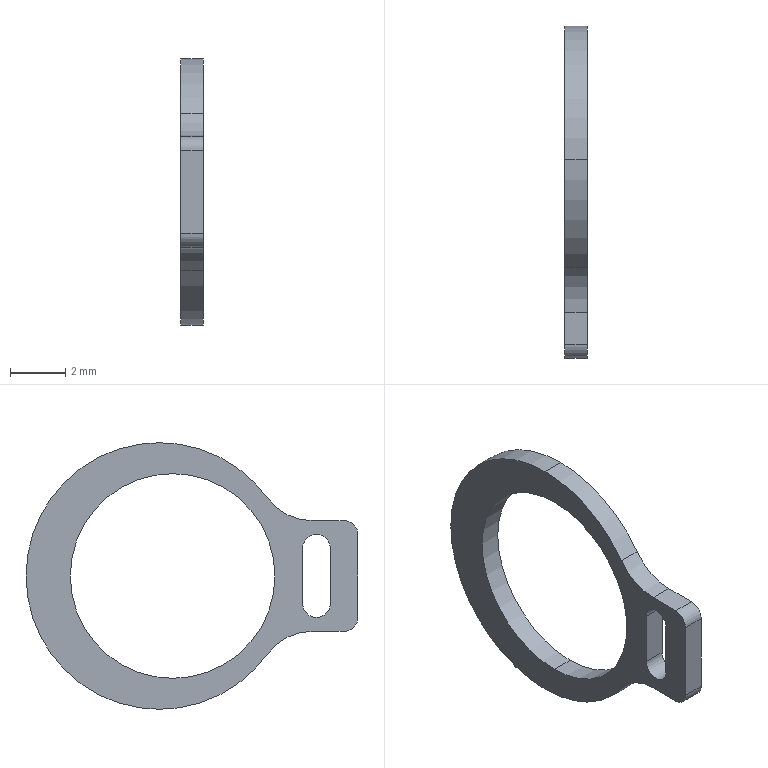Part | STEP file | 11-STWN811 | 1 solid | 19 faces | box 0.8 x 12 x 9.64 mm | volume 29.975 mm3 | cylinder 12 | plane 7 | commonest cylinder face diameters 1 x5 9.64 x3 4 x2 7.4 x2
STEP:
#1=CARTESIAN_POINT('',(0.4,0.,3.7));
#2=VERTEX_POINT('',#1);
#3=CARTESIAN_POINT('',(0.4,0.,-3.7));
#4=VERTEX_POINT('',#3);
#5=CARTESIAN_POINT('',(0.4,0.,0.));
#6=DIRECTION('',(1.,0.,0.));
#7=DIRECTION('',(0.,0.,-1.));
#8=AXIS2_PLACEMENT_3D('',#5,#6,#7);
#9=CIRCLE('',#8,3.7);
#10=EDGE_CURVE('',#2,#4,#9,.T.);
#11=ORIENTED_EDGE('',*,*,#10,.T.);
#12=CARTESIAN_POINT('',(-0.4,0.,-3.7));
#13=VERTEX_POINT('',#12);
#14=CARTESIAN_POINT('',(0.4,0.,-3.7));
#15=DIRECTION('',(-1.,0.,0.));
#16=VECTOR('',#15,1000.);
#17=LINE('',#14,#16);
#18=EDGE_CURVE('',#4,#13,#17,.T.);
#19=ORIENTED_EDGE('',*,*,#18,.T.);
#20=CARTESIAN_POINT('',(-0.4,0.,3.7));
#21=VERTEX_POINT('',#20);
#22=CARTESIAN_POINT('',(-0.4,0.,0.));
#23=DIRECTION('',(1.,0.,0.));
#24=DIRECTION('',(0.,0.,-1.));
#25=AXIS2_PLACEMENT_3D('',#22,#23,#24);
#26=CIRCLE('',#25,3.7);
#27=EDGE_CURVE('',#21,#13,#26,.T.);
#28=ORIENTED_EDGE('',*,*,#27,.F.);
#29=CARTESIAN_POINT('',(0.4,0.,3.7));
#30=DIRECTION('',(-1.,0.,0.));
#31=VECTOR('',#30,1000.);
#32=LINE('',#29,#31);
#33=EDGE_CURVE('',#2,#21,#32,.T.);
#34=ORIENTED_EDGE('',*,*,#33,.F.);
#35=EDGE_LOOP('',(#11,#19,#28,#34));
#36=FACE_OUTER_BOUND('',#35,.T.);
#37=CARTESIAN_POINT('',(0.4,0.,0.));
#38=DIRECTION('',(-1.,0.,0.));
#39=DIRECTION('',(0.,0.,1.));
#40=AXIS2_PLACEMENT_3D('',#37,#38,#39);
#41=CYLINDRICAL_SURFACE('',#40,3.7);
#42=ADVANCED_FACE('',(#36),#41,.F.);
#43=CARTESIAN_POINT('',(0.4,-4.7,1.));
#44=VERTEX_POINT('',#43);
#45=CARTESIAN_POINT('',(0.4,-5.2,1.5));
#46=VERTEX_POINT('',#45);
#47=CARTESIAN_POINT('',(0.4,-5.2,1.));
#48=DIRECTION('',(1.,0.,0.));
#49=DIRECTION('',(0.,0.,-1.));
#50=AXIS2_PLACEMENT_3D('',#47,#48,#49);
#51=CIRCLE('',#50,0.5);
#52=EDGE_CURVE('',#44,#46,#51,.T.);
#53=ORIENTED_EDGE('',*,*,#52,.T.);
#54=CARTESIAN_POINT('',(-0.4,-5.2,1.5));
#55=VERTEX_POINT('',#54);
#56=CARTESIAN_POINT('',(0.4,-5.2,1.5));
#57=DIRECTION('',(-1.,0.,0.));
#58=VECTOR('',#57,1000.);
#59=LINE('',#56,#58);
#60=EDGE_CURVE('',#46,#55,#59,.T.);
#61=ORIENTED_EDGE('',*,*,#60,.T.);
#62=CARTESIAN_POINT('',(-0.4,-4.7,1.));
#63=VERTEX_POINT('',#62);
#64=CARTESIAN_POINT('',(-0.4,-5.2,1.));
#65=DIRECTION('',(1.,0.,0.));
#66=DIRECTION('',(0.,0.,-1.));
#67=AXIS2_PLACEMENT_3D('',#64,#65,#66);
#68=CIRCLE('',#67,0.5);
#69=EDGE_CURVE('',#63,#55,#68,.T.);
#70=ORIENTED_EDGE('',*,*,#69,.F.);
#71=CARTESIAN_POINT('',(0.4,-4.7,1.));
#72=DIRECTION('',(-1.,0.,0.));
#73=VECTOR('',#72,1000.);
#74=LINE('',#71,#73);
#75=EDGE_CURVE('',#44,#63,#74,.T.);
#76=ORIENTED_EDGE('',*,*,#75,.F.);
#77=EDGE_LOOP('',(#53,#61,#70,#76));
#78=FACE_OUTER_BOUND('',#77,.T.);
#79=CARTESIAN_POINT('',(0.4,-5.2,1.));
#80=DIRECTION('',(-1.,0.,0.));
#81=DIRECTION('',(0.,0.,1.));
#82=AXIS2_PLACEMENT_3D('',#79,#80,#81);
#83=CYLINDRICAL_SURFACE('',#82,0.5);
#84=ADVANCED_FACE('',(#78),#83,.F.);
#85=CARTESIAN_POINT('',(0.4,0.48,-4.82));
#86=VERTEX_POINT('',#85);
#87=CARTESIAN_POINT('',(0.4,0.48,4.82));
#88=VERTEX_POINT('',#87);
#89=CARTESIAN_POINT('',(0.4,0.48,0.));
#90=DIRECTION('',(1.,0.,0.));
#91=DIRECTION('',(0.,0.,-1.));
#92=AXIS2_PLACEMENT_3D('',#89,#90,#91);
#93=CIRCLE('',#92,4.82);
#94=EDGE_CURVE('',#86,#88,#93,.T.);
#95=ORIENTED_EDGE('',*,*,#94,.F.);
#96=CARTESIAN_POINT('',(-0.4,0.48,-4.82));
#97=VERTEX_POINT('',#96);
#98=CARTESIAN_POINT('',(0.4,0.48,-4.82));
#99=DIRECTION('',(-1.,0.,0.));
#100=VECTOR('',#99,1000.);
#101=LINE('',#98,#100);
#102=EDGE_CURVE('',#86,#97,#101,.T.);
#103=ORIENTED_EDGE('',*,*,#102,.T.);
#104=CARTESIAN_POINT('',(-0.4,0.48,4.82));
#105=VERTEX_POINT('',#104);
#106=CARTESIAN_POINT('',(-0.4,0.48,0.));
#107=DIRECTION('',(1.,0.,0.));
#108=DIRECTION('',(0.,0.,-1.));
#109=AXIS2_PLACEMENT_3D('',#106,#107,#108);
#110=CIRCLE('',#109,4.82);
#111=EDGE_CURVE('',#97,#105,#110,.T.);
#112=ORIENTED_EDGE('',*,*,#111,.T.);
#113=CARTESIAN_POINT('',(0.4,0.48,4.82));
#114=DIRECTION('',(-1.,0.,0.));
#115=VECTOR('',#114,1000.);
#116=LINE('',#113,#115);
#117=EDGE_CURVE('',#88,#105,#116,.T.);
#118=ORIENTED_EDGE('',*,*,#117,.F.);
#119=EDGE_LOOP('',(#95,#103,#112,#118));
#120=FACE_OUTER_BOUND('',#119,.T.);
#121=CARTESIAN_POINT('',(0.4,0.48,0.));
#122=DIRECTION('',(-1.,0.,0.));
#123=DIRECTION('',(0.,0.,1.));
#124=AXIS2_PLACEMENT_3D('',#121,#122,#123);
#125=CYLINDRICAL_SURFACE('',#124,4.82);
#126=ADVANCED_FACE('',(#120),#125,.T.);
#127=CARTESIAN_POINT('',(0.4,-3.424,2.827));
#128=VERTEX_POINT('',#127);
#129=CARTESIAN_POINT('',(0.4,0.48,0.));
#130=DIRECTION('',(1.,0.,0.));
#131=DIRECTION('',(0.,0.,-1.));
#132=AXIS2_PLACEMENT_3D('',#129,#130,#131);
#133=CIRCLE('',#132,4.82);
#134=EDGE_CURVE('',#88,#128,#133,.T.);
#135=ORIENTED_EDGE('',*,*,#134,.F.);
#136=ORIENTED_EDGE('',*,*,#117,.T.);
#137=CARTESIAN_POINT('',(-0.4,-3.424,2.827));
#138=VERTEX_POINT('',#137);
#139=CARTESIAN_POINT('',(-0.4,0.48,0.));
#140=DIRECTION('',(1.,0.,0.));
#141=DIRECTION('',(0.,0.,-1.));
#142=AXIS2_PLACEMENT_3D('',#139,#140,#141);
#143=CIRCLE('',#142,4.82);
#144=EDGE_CURVE('',#105,#138,#143,.T.);
#145=ORIENTED_EDGE('',*,*,#144,.T.);
#146=CARTESIAN_POINT('',(0.4,-3.424,2.827));
#147=DIRECTION('',(-1.,0.,0.));
#148=VECTOR('',#147,1000.);
#149=LINE('',#146,#148);
#150=EDGE_CURVE('',#128,#138,#149,.T.);
#151=ORIENTED_EDGE('',*,*,#150,.F.);
#152=EDGE_LOOP('',(#135,#136,#145,#151));
#153=FACE_OUTER_BOUND('',#152,.T.);
#154=CARTESIAN_POINT('',(0.4,0.48,0.));
#155=DIRECTION('',(-1.,0.,0.));
#156=DIRECTION('',(0.,0.,1.));
#157=AXIS2_PLACEMENT_3D('',#154,#155,#156);
#158=CYLINDRICAL_SURFACE('',#157,4.82);
#159=ADVANCED_FACE('',(#153),#158,.T.);
#160=ORIENTED_EDGE('',*,*,#52,.F.);
#161=CARTESIAN_POINT('',(0.4,-4.7,-1.));
#162=VERTEX_POINT('',#161);
#163=CARTESIAN_POINT('',(0.4,-4.7,-1.));
#164=DIRECTION('',(0.,0.,1.));
#165=VECTOR('',#164,1000.);
#166=LINE('',#163,#165);
#167=EDGE_CURVE('',#162,#44,#166,.T.);
#168=ORIENTED_EDGE('',*,*,#167,.F.);
#169=CARTESIAN_POINT('',(0.4,-5.7,-1.));
#170=VERTEX_POINT('',#169);
#171=CARTESIAN_POINT('',(0.4,-5.2,-1.));
#172=DIRECTION('',(1.,0.,0.));
#173=DIRECTION('',(0.,0.,-1.));
#174=AXIS2_PLACEMENT_3D('',#171,#172,#173);
#175=CIRCLE('',#174,0.5);
#176=EDGE_CURVE('',#170,#162,#175,.T.);
#177=ORIENTED_EDGE('',*,*,#176,.F.);
#178=CARTESIAN_POINT('',(0.4,-5.7,1.));
#179=VERTEX_POINT('',#178);
#180=CARTESIAN_POINT('',(0.4,-5.7,1.));
#181=DIRECTION('',(0.,0.,-1.));
#182=VECTOR('',#181,1000.);
#183=LINE('',#180,#182);
#184=EDGE_CURVE('',#179,#170,#183,.T.);
#185=ORIENTED_EDGE('',*,*,#184,.F.);
#186=CARTESIAN_POINT('',(0.4,-5.2,1.));
#187=DIRECTION('',(1.,0.,0.));
#188=DIRECTION('',(0.,0.,-1.));
#189=AXIS2_PLACEMENT_3D('',#186,#187,#188);
#190=CIRCLE('',#189,0.5);
#191=EDGE_CURVE('',#46,#179,#190,.T.);
#192=ORIENTED_EDGE('',*,*,#191,.F.);
#193=EDGE_LOOP('',(#160,#168,#177,#185,#192));
#194=FACE_BOUND('',#193,.T.);
#195=CARTESIAN_POINT('',(0.4,-5.044,-2.));
#196=VERTEX_POINT('',#195);
#197=CARTESIAN_POINT('',(0.4,-3.424,-2.827));
#198=VERTEX_POINT('',#197);
#199=CARTESIAN_POINT('',(0.4,-5.044,-4.));
#200=DIRECTION('',(-1.,0.,0.));
#201=DIRECTION('',(0.,0.,1.));
#202=AXIS2_PLACEMENT_3D('',#199,#200,#201);
#203=CIRCLE('',#202,2.);
#204=EDGE_CURVE('',#196,#198,#203,.T.);
#205=ORIENTED_EDGE('',*,*,#204,.T.);
#206=CARTESIAN_POINT('',(0.4,0.48,0.));
#207=DIRECTION('',(1.,0.,0.));
#208=DIRECTION('',(0.,0.,-1.));
#209=AXIS2_PLACEMENT_3D('',#206,#207,#208);
#210=CIRCLE('',#209,4.82);
#211=EDGE_CURVE('',#198,#86,#210,.T.);
#212=ORIENTED_EDGE('',*,*,#211,.T.);
#213=ORIENTED_EDGE('',*,*,#94,.T.);
#214=ORIENTED_EDGE('',*,*,#134,.T.);
#215=CARTESIAN_POINT('',(0.4,-5.044,2.));
#216=VERTEX_POINT('',#215);
#217=CARTESIAN_POINT('',(0.4,-5.044,4.));
#218=DIRECTION('',(-1.,0.,0.));
#219=DIRECTION('',(0.,0.,1.));
#220=AXIS2_PLACEMENT_3D('',#217,#218,#219);
#221=CIRCLE('',#220,2.);
#222=EDGE_CURVE('',#128,#216,#221,.T.);
#223=ORIENTED_EDGE('',*,*,#222,.T.);
#224=CARTESIAN_POINT('',(0.4,-6.2,2.));
#225=VERTEX_POINT('',#224);
#226=CARTESIAN_POINT('',(0.4,-5.044,2.));
#227=DIRECTION('',(0.,-1.,0.));
#228=VECTOR('',#227,1000.);
#229=LINE('',#226,#228);
#230=EDGE_CURVE('',#216,#225,#229,.T.);
#231=ORIENTED_EDGE('',*,*,#230,.T.);
#232=CARTESIAN_POINT('',(0.4,-6.7,1.5));
#233=VERTEX_POINT('',#232);
#234=CARTESIAN_POINT('',(0.4,-6.2,1.5));
#235=DIRECTION('',(1.,0.,0.));
#236=DIRECTION('',(0.,0.,-1.));
#237=AXIS2_PLACEMENT_3D('',#234,#235,#236);
#238=CIRCLE('',#237,0.5);
#239=EDGE_CURVE('',#225,#233,#238,.T.);
#240=ORIENTED_EDGE('',*,*,#239,.T.);
#241=CARTESIAN_POINT('',(0.4,-6.7,-1.5));
#242=VERTEX_POINT('',#241);
#243=CARTESIAN_POINT('',(0.4,-6.7,1.5));
#244=DIRECTION('',(0.,0.,-1.));
#245=VECTOR('',#244,1000.);
#246=LINE('',#243,#245);
#247=EDGE_CURVE('',#233,#242,#246,.T.);
#248=ORIENTED_EDGE('',*,*,#247,.T.);
#249=CARTESIAN_POINT('',(0.4,-6.2,-2.));
#250=VERTEX_POINT('',#249);
#251=CARTESIAN_POINT('',(0.4,-6.2,-1.5));
#252=DIRECTION('',(1.,0.,0.));
#253=DIRECTION('',(0.,0.,-1.));
#254=AXIS2_PLACEMENT_3D('',#251,#252,#253);
#255=CIRCLE('',#254,0.5);
#256=EDGE_CURVE('',#242,#250,#255,.T.);
#257=ORIENTED_EDGE('',*,*,#256,.T.);
#258=CARTESIAN_POINT('',(0.4,-6.2,-2.));
#259=DIRECTION('',(0.,1.,0.));
#260=VECTOR('',#259,1000.);
#261=LINE('',#258,#260);
#262=EDGE_CURVE('',#250,#196,#261,.T.);
#263=ORIENTED_EDGE('',*,*,#262,.T.);
#264=EDGE_LOOP('',(#205,#212,#213,#214,#223,#231,#240,#248,#257,#263));
#265=FACE_OUTER_BOUND('',#264,.T.);
#266=ORIENTED_EDGE('',*,*,#10,.F.);
#267=CARTESIAN_POINT('',(0.4,0.,0.));
#268=DIRECTION('',(1.,0.,0.));
#269=DIRECTION('',(0.,0.,-1.));
#270=AXIS2_PLACEMENT_3D('',#267,#268,#269);
#271=CIRCLE('',#270,3.7);
#272=EDGE_CURVE('',#4,#2,#271,.T.);
#273=ORIENTED_EDGE('',*,*,#272,.F.);
#274=EDGE_LOOP('',(#266,#273));
#275=FACE_BOUND('',#274,.T.);
#276=CARTESIAN_POINT('',(0.4,-5.044,-4.));
#277=DIRECTION('',(-1.,0.,0.));
#278=DIRECTION('',(0.,0.,1.));
#279=AXIS2_PLACEMENT_3D('',#276,#277,#278);
#280=PLANE('',#279);
#281=ADVANCED_FACE('',(#194,#265,#275),#280,.F.);
#282=CARTESIAN_POINT('',(-0.4,-5.044,-2.));
#283=VERTEX_POINT('',#282);
#284=CARTESIAN_POINT('',(0.4,-5.044,-2.));
#285=DIRECTION('',(-1.,0.,0.));
#286=VECTOR('',#285,1000.);
#287=LINE('',#284,#286);
#288=EDGE_CURVE('',#196,#283,#287,.T.);
#289=ORIENTED_EDGE('',*,*,#288,.T.);
#290=CARTESIAN_POINT('',(-0.4,-3.424,-2.827));
#291=VERTEX_POINT('',#290);
#292=CARTESIAN_POINT('',(-0.4,-5.044,-4.));
#293=DIRECTION('',(-1.,0.,0.));
#294=DIRECTION('',(0.,0.,1.));
#295=AXIS2_PLACEMENT_3D('',#292,#293,#294);
#296=CIRCLE('',#295,2.);
#297=EDGE_CURVE('',#283,#291,#296,.T.);
#298=ORIENTED_EDGE('',*,*,#297,.T.);
#299=CARTESIAN_POINT('',(0.4,-3.424,-2.827));
#300=DIRECTION('',(-1.,0.,0.));
#301=VECTOR('',#300,1000.);
#302=LINE('',#299,#301);
#303=EDGE_CURVE('',#198,#291,#302,.T.);
#304=ORIENTED_EDGE('',*,*,#303,.F.);
#305=ORIENTED_EDGE('',*,*,#204,.F.);
#306=EDGE_LOOP('',(#289,#298,#304,#305));
#307=FACE_OUTER_BOUND('',#306,.T.);
#308=CARTESIAN_POINT('',(0.4,-5.044,-4.));
#309=DIRECTION('',(-1.,0.,0.));
#310=DIRECTION('',(0.,0.,1.));
#311=AXIS2_PLACEMENT_3D('',#308,#309,#310);
#312=CYLINDRICAL_SURFACE('',#311,2.);
#313=ADVANCED_FACE('',(#307),#312,.F.);
#314=ORIENTED_EDGE('',*,*,#102,.F.);
#315=ORIENTED_EDGE('',*,*,#211,.F.);
#316=ORIENTED_EDGE('',*,*,#303,.T.);
#317=CARTESIAN_POINT('',(-0.4,0.48,0.));
#318=DIRECTION('',(1.,0.,0.));
#319=DIRECTION('',(0.,0.,-1.));
#320=AXIS2_PLACEMENT_3D('',#317,#318,#319);
#321=CIRCLE('',#320,4.82);
#322=EDGE_CURVE('',#291,#97,#321,.T.);
#323=ORIENTED_EDGE('',*,*,#322,.T.);
#324=EDGE_LOOP('',(#314,#315,#316,#323));
#325=FACE_OUTER_BOUND('',#324,.T.);
#326=CARTESIAN_POINT('',(0.4,0.48,0.));
#327=DIRECTION('',(-1.,0.,0.));
#328=DIRECTION('',(0.,0.,1.));
#329=AXIS2_PLACEMENT_3D('',#326,#327,#328);
#330=CYLINDRICAL_SURFACE('',#329,4.82);
#331=ADVANCED_FACE('',(#325),#330,.T.);
#332=ORIENTED_EDGE('',*,*,#150,.T.);
#333=CARTESIAN_POINT('',(-0.4,-5.044,2.));
#334=VERTEX_POINT('',#333);
#335=CARTESIAN_POINT('',(-0.4,-5.044,4.));
#336=DIRECTION('',(-1.,0.,0.));
#337=DIRECTION('',(0.,0.,1.));
#338=AXIS2_PLACEMENT_3D('',#335,#336,#337);
#339=CIRCLE('',#338,2.);
#340=EDGE_CURVE('',#138,#334,#339,.T.);
#341=ORIENTED_EDGE('',*,*,#340,.T.);
#342=CARTESIAN_POINT('',(0.4,-5.044,2.));
#343=DIRECTION('',(-1.,0.,0.));
#344=VECTOR('',#343,1000.);
#345=LINE('',#342,#344);
#346=EDGE_CURVE('',#216,#334,#345,.T.);
#347=ORIENTED_EDGE('',*,*,#346,.F.);
#348=ORIENTED_EDGE('',*,*,#222,.F.);
#349=EDGE_LOOP('',(#332,#341,#347,#348));
#350=FACE_OUTER_BOUND('',#349,.T.);
#351=CARTESIAN_POINT('',(0.4,-5.044,4.));
#352=DIRECTION('',(-1.,0.,0.));
#353=DIRECTION('',(0.,0.,1.));
#354=AXIS2_PLACEMENT_3D('',#351,#352,#353);
#355=CYLINDRICAL_SURFACE('',#354,2.);
#356=ADVANCED_FACE('',(#350),#355,.F.);
#357=ORIENTED_EDGE('',*,*,#346,.T.);
#358=CARTESIAN_POINT('',(-0.4,-6.2,2.));
#359=VERTEX_POINT('',#358);
#360=CARTESIAN_POINT('',(-0.4,-5.044,2.));
#361=DIRECTION('',(0.,-1.,0.));
#362=VECTOR('',#361,1000.);
#363=LINE('',#360,#362);
#364=EDGE_CURVE('',#334,#359,#363,.T.);
#365=ORIENTED_EDGE('',*,*,#364,.T.);
#366=CARTESIAN_POINT('',(0.4,-6.2,2.));
#367=DIRECTION('',(-1.,0.,0.));
#368=VECTOR('',#367,1000.);
#369=LINE('',#366,#368);
#370=EDGE_CURVE('',#225,#359,#369,.T.);
#371=ORIENTED_EDGE('',*,*,#370,.F.);
#372=ORIENTED_EDGE('',*,*,#230,.F.);
#373=EDGE_LOOP('',(#357,#365,#371,#372));
#374=FACE_OUTER_BOUND('',#373,.T.);
#375=CARTESIAN_POINT('',(0.4,-5.044,2.));
#376=DIRECTION('',(0.,0.,-1.));
#377=DIRECTION('',(-1.,0.,0.));
#378=AXIS2_PLACEMENT_3D('',#375,#376,#377);
#379=PLANE('',#378);
#380=ADVANCED_FACE('',(#374),#379,.F.);
#381=ORIENTED_EDGE('',*,*,#370,.T.);
#382=CARTESIAN_POINT('',(-0.4,-6.7,1.5));
#383=VERTEX_POINT('',#382);
#384=CARTESIAN_POINT('',(-0.4,-6.2,1.5));
#385=DIRECTION('',(1.,0.,0.));
#386=DIRECTION('',(0.,0.,-1.));
#387=AXIS2_PLACEMENT_3D('',#384,#385,#386);
#388=CIRCLE('',#387,0.5);
#389=EDGE_CURVE('',#359,#383,#388,.T.);
#390=ORIENTED_EDGE('',*,*,#389,.T.);
#391=CARTESIAN_POINT('',(0.4,-6.7,1.5));
#392=DIRECTION('',(-1.,0.,0.));
#393=VECTOR('',#392,1000.);
#394=LINE('',#391,#393);
#395=EDGE_CURVE('',#233,#383,#394,.T.);
#396=ORIENTED_EDGE('',*,*,#395,.F.);
#397=ORIENTED_EDGE('',*,*,#239,.F.);
#398=EDGE_LOOP('',(#381,#390,#396,#397));
#399=FACE_OUTER_BOUND('',#398,.T.);
#400=CARTESIAN_POINT('',(0.4,-6.2,1.5));
#401=DIRECTION('',(-1.,0.,0.));
#402=DIRECTION('',(0.,0.,1.));
#403=AXIS2_PLACEMENT_3D('',#400,#401,#402);
#404=CYLINDRICAL_SURFACE('',#403,0.5);
#405=ADVANCED_FACE('',(#399),#404,.T.);
#406=ORIENTED_EDGE('',*,*,#395,.T.);
#407=CARTESIAN_POINT('',(-0.4,-6.7,-1.5));
#408=VERTEX_POINT('',#407);
#409=CARTESIAN_POINT('',(-0.4,-6.7,1.5));
#410=DIRECTION('',(0.,0.,-1.));
#411=VECTOR('',#410,1000.);
#412=LINE('',#409,#411);
#413=EDGE_CURVE('',#383,#408,#412,.T.);
#414=ORIENTED_EDGE('',*,*,#413,.T.);
#415=CARTESIAN_POINT('',(0.4,-6.7,-1.5));
#416=DIRECTION('',(-1.,0.,0.));
#417=VECTOR('',#416,1000.);
#418=LINE('',#415,#417);
#419=EDGE_CURVE('',#242,#408,#418,.T.);
#420=ORIENTED_EDGE('',*,*,#419,.F.);
#421=ORIENTED_EDGE('',*,*,#247,.F.);
#422=EDGE_LOOP('',(#406,#414,#420,#421));
#423=FACE_OUTER_BOUND('',#422,.T.);
#424=CARTESIAN_POINT('',(0.4,-6.7,1.5));
#425=DIRECTION('',(0.,1.,0.));
#426=DIRECTION('',(0.,0.,1.));
#427=AXIS2_PLACEMENT_3D('',#424,#425,#426);
#428=PLANE('',#427);
#429=ADVANCED_FACE('',(#423),#428,.F.);
#430=ORIENTED_EDGE('',*,*,#419,.T.);
#431=CARTESIAN_POINT('',(-0.4,-6.2,-2.));
#432=VERTEX_POINT('',#431);
#433=CARTESIAN_POINT('',(-0.4,-6.2,-1.5));
#434=DIRECTION('',(1.,0.,0.));
#435=DIRECTION('',(0.,0.,-1.));
#436=AXIS2_PLACEMENT_3D('',#433,#434,#435);
#437=CIRCLE('',#436,0.5);
#438=EDGE_CURVE('',#408,#432,#437,.T.);
#439=ORIENTED_EDGE('',*,*,#438,.T.);
#440=CARTESIAN_POINT('',(0.4,-6.2,-2.));
#441=DIRECTION('',(-1.,0.,0.));
#442=VECTOR('',#441,1000.);
#443=LINE('',#440,#442);
#444=EDGE_CURVE('',#250,#432,#443,.T.);
#445=ORIENTED_EDGE('',*,*,#444,.F.);
#446=ORIENTED_EDGE('',*,*,#256,.F.);
#447=EDGE_LOOP('',(#430,#439,#445,#446));
#448=FACE_OUTER_BOUND('',#447,.T.);
#449=CARTESIAN_POINT('',(0.4,-6.2,-1.5));
#450=DIRECTION('',(-1.,0.,0.));
#451=DIRECTION('',(0.,0.,1.));
#452=AXIS2_PLACEMENT_3D('',#449,#450,#451);
#453=CYLINDRICAL_SURFACE('',#452,0.5);
#454=ADVANCED_FACE('',(#448),#453,.T.);
#455=ORIENTED_EDGE('',*,*,#444,.T.);
#456=CARTESIAN_POINT('',(-0.4,-6.2,-2.));
#457=DIRECTION('',(0.,1.,0.));
#458=VECTOR('',#457,1000.);
#459=LINE('',#456,#458);
#460=EDGE_CURVE('',#432,#283,#459,.T.);
#461=ORIENTED_EDGE('',*,*,#460,.T.);
#462=ORIENTED_EDGE('',*,*,#288,.F.);
#463=ORIENTED_EDGE('',*,*,#262,.F.);
#464=EDGE_LOOP('',(#455,#461,#462,#463));
#465=FACE_OUTER_BOUND('',#464,.T.);
#466=CARTESIAN_POINT('',(0.4,-6.2,-2.));
#467=DIRECTION('',(0.,0.,1.));
#468=DIRECTION('',(1.,0.,0.));
#469=AXIS2_PLACEMENT_3D('',#466,#467,#468);
#470=PLANE('',#469);
#471=ADVANCED_FACE('',(#465),#470,.F.);
#472=ORIENTED_EDGE('',*,*,#60,.F.);
#473=ORIENTED_EDGE('',*,*,#191,.T.);
#474=CARTESIAN_POINT('',(-0.4,-5.7,1.));
#475=VERTEX_POINT('',#474);
#476=CARTESIAN_POINT('',(0.4,-5.7,1.));
#477=DIRECTION('',(-1.,0.,0.));
#478=VECTOR('',#477,1000.);
#479=LINE('',#476,#478);
#480=EDGE_CURVE('',#179,#475,#479,.T.);
#481=ORIENTED_EDGE('',*,*,#480,.T.);
#482=CARTESIAN_POINT('',(-0.4,-5.2,1.));
#483=DIRECTION('',(1.,0.,0.));
#484=DIRECTION('',(0.,0.,-1.));
#485=AXIS2_PLACEMENT_3D('',#482,#483,#484);
#486=CIRCLE('',#485,0.5);
#487=EDGE_CURVE('',#55,#475,#486,.T.);
#488=ORIENTED_EDGE('',*,*,#487,.F.);
#489=EDGE_LOOP('',(#472,#473,#481,#488));
#490=FACE_OUTER_BOUND('',#489,.T.);
#491=CARTESIAN_POINT('',(0.4,-5.2,1.));
#492=DIRECTION('',(-1.,0.,0.));
#493=DIRECTION('',(0.,0.,1.));
#494=AXIS2_PLACEMENT_3D('',#491,#492,#493);
#495=CYLINDRICAL_SURFACE('',#494,0.5);
#496=ADVANCED_FACE('',(#490),#495,.F.);
#497=CARTESIAN_POINT('',(-0.4,-5.7,-1.));
#498=VERTEX_POINT('',#497);
#499=CARTESIAN_POINT('',(0.4,-5.7,-1.));
#500=DIRECTION('',(-1.,0.,0.));
#501=VECTOR('',#500,1000.);
#502=LINE('',#499,#501);
#503=EDGE_CURVE('',#170,#498,#502,.T.);
#504=ORIENTED_EDGE('',*,*,#503,.T.);
#505=CARTESIAN_POINT('',(-0.4,-5.7,1.));
#506=DIRECTION('',(0.,0.,-1.));
#507=VECTOR('',#506,1000.);
#508=LINE('',#505,#507);
#509=EDGE_CURVE('',#475,#498,#508,.T.);
#510=ORIENTED_EDGE('',*,*,#509,.F.);
#511=ORIENTED_EDGE('',*,*,#480,.F.);
#512=ORIENTED_EDGE('',*,*,#184,.T.);
#513=EDGE_LOOP('',(#504,#510,#511,#512));
#514=FACE_OUTER_BOUND('',#513,.T.);
#515=CARTESIAN_POINT('',(0.4,-5.7,1.));
#516=DIRECTION('',(0.,1.,0.));
#517=DIRECTION('',(0.,0.,1.));
#518=AXIS2_PLACEMENT_3D('',#515,#516,#517);
#519=PLANE('',#518);
#520=ADVANCED_FACE('',(#514),#519,.T.);
#521=CARTESIAN_POINT('',(-0.4,-4.7,-1.));
#522=VERTEX_POINT('',#521);
#523=CARTESIAN_POINT('',(0.4,-4.7,-1.));
#524=DIRECTION('',(-1.,0.,0.));
#525=VECTOR('',#524,1000.);
#526=LINE('',#523,#525);
#527=EDGE_CURVE('',#162,#522,#526,.T.);
#528=ORIENTED_EDGE('',*,*,#527,.T.);
#529=CARTESIAN_POINT('',(-0.4,-5.2,-1.));
#530=DIRECTION('',(1.,0.,0.));
#531=DIRECTION('',(0.,0.,-1.));
#532=AXIS2_PLACEMENT_3D('',#529,#530,#531);
#533=CIRCLE('',#532,0.5);
#534=EDGE_CURVE('',#498,#522,#533,.T.);
#535=ORIENTED_EDGE('',*,*,#534,.F.);
#536=ORIENTED_EDGE('',*,*,#503,.F.);
#537=ORIENTED_EDGE('',*,*,#176,.T.);
#538=EDGE_LOOP('',(#528,#535,#536,#537));
#539=FACE_OUTER_BOUND('',#538,.T.);
#540=CARTESIAN_POINT('',(0.4,-5.2,-1.));
#541=DIRECTION('',(-1.,0.,0.));
#542=DIRECTION('',(0.,0.,1.));
#543=AXIS2_PLACEMENT_3D('',#540,#541,#542);
#544=CYLINDRICAL_SURFACE('',#543,0.5);
#545=ADVANCED_FACE('',(#539),#544,.F.);
#546=ORIENTED_EDGE('',*,*,#75,.T.);
#547=CARTESIAN_POINT('',(-0.4,-4.7,-1.));
#548=DIRECTION('',(0.,0.,1.));
#549=VECTOR('',#548,1000.);
#550=LINE('',#547,#549);
#551=EDGE_CURVE('',#522,#63,#550,.T.);
#552=ORIENTED_EDGE('',*,*,#551,.F.);
#553=ORIENTED_EDGE('',*,*,#527,.F.);
#554=ORIENTED_EDGE('',*,*,#167,.T.);
#555=EDGE_LOOP('',(#546,#552,#553,#554));
#556=FACE_OUTER_BOUND('',#555,.T.);
#557=CARTESIAN_POINT('',(0.4,-4.7,-1.));
#558=DIRECTION('',(0.,-1.,0.));
#559=DIRECTION('',(0.,0.,-1.));
#560=AXIS2_PLACEMENT_3D('',#557,#558,#559);
#561=PLANE('',#560);
#562=ADVANCED_FACE('',(#556),#561,.T.);
#563=ORIENTED_EDGE('',*,*,#18,.F.);
#564=ORIENTED_EDGE('',*,*,#272,.T.);
#565=ORIENTED_EDGE('',*,*,#33,.T.);
#566=CARTESIAN_POINT('',(-0.4,0.,0.));
#567=DIRECTION('',(1.,0.,0.));
#568=DIRECTION('',(0.,0.,-1.));
#569=AXIS2_PLACEMENT_3D('',#566,#567,#568);
#570=CIRCLE('',#569,3.7);
#571=EDGE_CURVE('',#13,#21,#570,.T.);
#572=ORIENTED_EDGE('',*,*,#571,.F.);
#573=EDGE_LOOP('',(#563,#564,#565,#572));
#574=FACE_OUTER_BOUND('',#573,.T.);
#575=CARTESIAN_POINT('',(0.4,0.,0.));
#576=DIRECTION('',(-1.,0.,0.));
#577=DIRECTION('',(0.,0.,1.));
#578=AXIS2_PLACEMENT_3D('',#575,#576,#577);
#579=CYLINDRICAL_SURFACE('',#578,3.7);
#580=ADVANCED_FACE('',(#574),#579,.F.);
#581=ORIENTED_EDGE('',*,*,#27,.T.);
#582=ORIENTED_EDGE('',*,*,#571,.T.);
#583=EDGE_LOOP('',(#581,#582));
#584=FACE_BOUND('',#583,.T.);
#585=ORIENTED_EDGE('',*,*,#69,.T.);
#586=ORIENTED_EDGE('',*,*,#487,.T.);
#587=ORIENTED_EDGE('',*,*,#509,.T.);
#588=ORIENTED_EDGE('',*,*,#534,.T.);
#589=ORIENTED_EDGE('',*,*,#551,.T.);
#590=EDGE_LOOP('',(#585,#586,#587,#588,#589));
#591=FACE_BOUND('',#590,.T.);
#592=ORIENTED_EDGE('',*,*,#297,.F.);
#593=ORIENTED_EDGE('',*,*,#460,.F.);
#594=ORIENTED_EDGE('',*,*,#438,.F.);
#595=ORIENTED_EDGE('',*,*,#413,.F.);
#596=ORIENTED_EDGE('',*,*,#389,.F.);
#597=ORIENTED_EDGE('',*,*,#364,.F.);
#598=ORIENTED_EDGE('',*,*,#340,.F.);
#599=ORIENTED_EDGE('',*,*,#144,.F.);
#600=ORIENTED_EDGE('',*,*,#111,.F.);
#601=ORIENTED_EDGE('',*,*,#322,.F.);
#602=EDGE_LOOP('',(#592,#593,#594,#595,#596,#597,#598,#599,#600,#601));
#603=FACE_OUTER_BOUND('',#602,.T.);
#604=CARTESIAN_POINT('',(-0.4,-5.044,-4.));
#605=DIRECTION('',(-1.,0.,0.));
#606=DIRECTION('',(0.,0.,1.));
#607=AXIS2_PLACEMENT_3D('',#604,#605,#606);
#608=PLANE('',#607);
#609=ADVANCED_FACE('',(#584,#591,#603),#608,.T.);
#610=CLOSED_SHELL('',(#42,#84,#126,#159,#281,#313,#331,#356,#380,#405,#429,#454,#471,#496,#520,#545,#562,#580,#609));
#611=MANIFOLD_SOLID_BREP('',#610);
#612=CARTESIAN_POINT('',(0.,0.,0.));
#613=DIRECTION('',(0.,0.,1.));
#614=DIRECTION('',(1.,0.,0.));
#615=AXIS2_PLACEMENT_3D('',#612,#613,#614);
#616=(LENGTH_UNIT()NAMED_UNIT(*)SI_UNIT(.MILLI.,.METRE.));
#617=UNCERTAINTY_MEASURE_WITH_UNIT(LENGTH_MEASURE(0.00001),#616,'','');
#618=(NAMED_UNIT(*)PLANE_ANGLE_UNIT()SI_UNIT($,.RADIAN.));
#619=(NAMED_UNIT(*)SI_UNIT($,.STERADIAN.)SOLID_ANGLE_UNIT());
#620=(GEOMETRIC_REPRESENTATION_CONTEXT(3)GLOBAL_UNCERTAINTY_ASSIGNED_CONTEXT((#617))GLOBAL_UNIT_ASSIGNED_CONTEXT((#616,#618,#619))REPRESENTATION_CONTEXT('',''));
#621=ADVANCED_BREP_SHAPE_REPRESENTATION('',(#611,#615),#620);